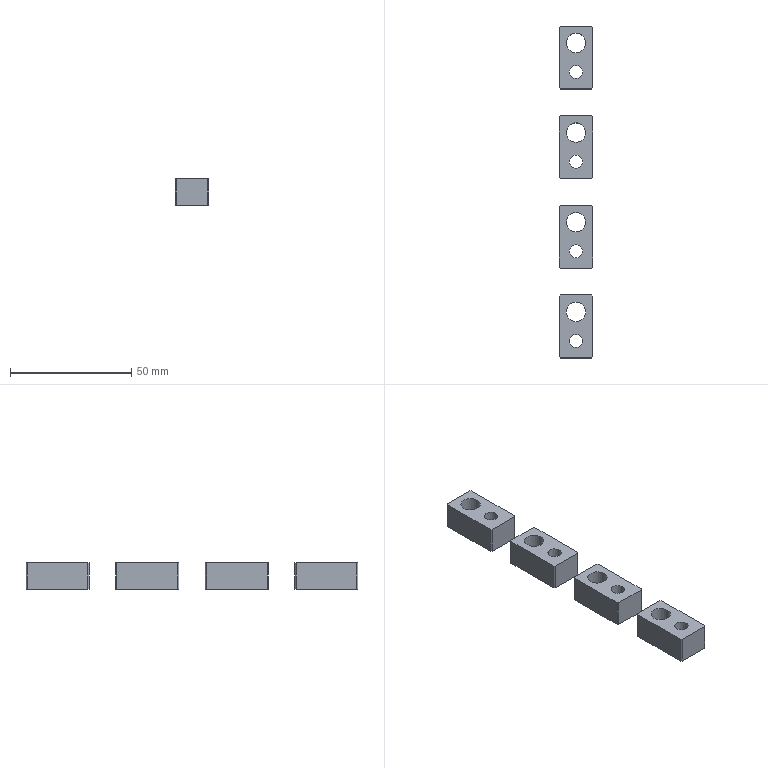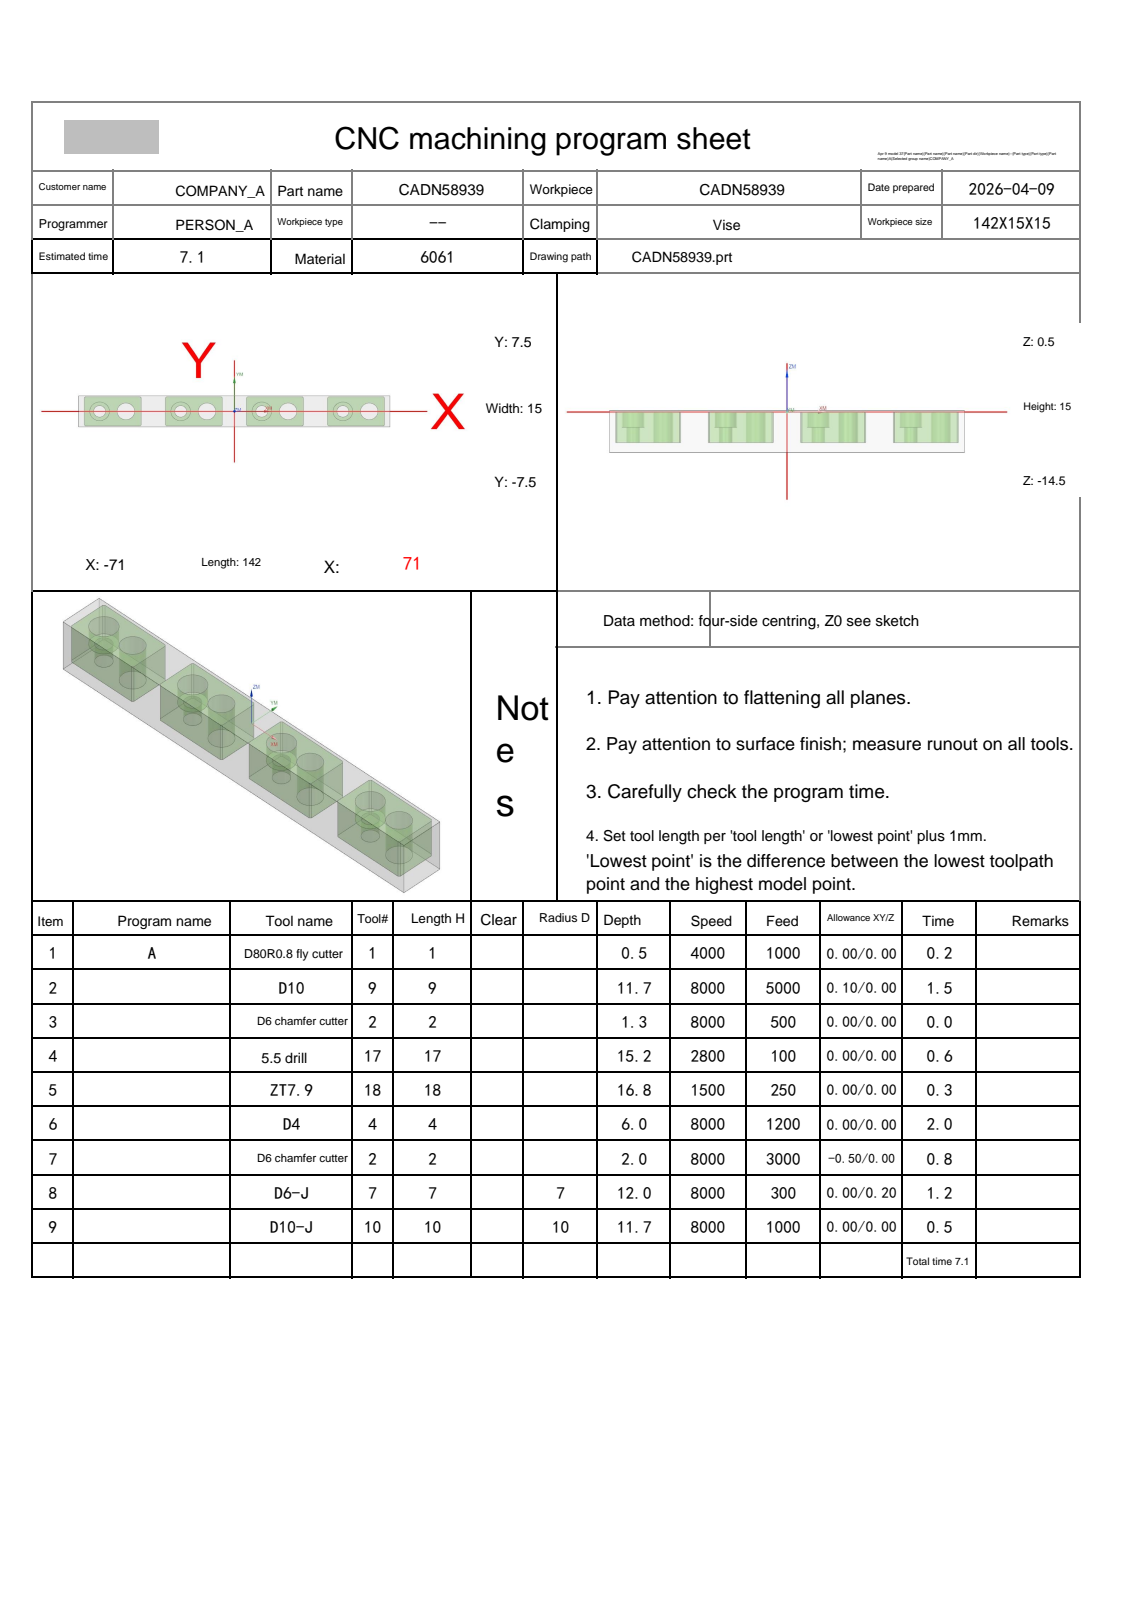NC program | NX | posted by the shop | part box 14 x 137 x 11 mm
Lines 1841 to 2072 of 2072:
N8 T07 M06
(D6-J  D=6. R=0. H=07 ce=0.00 di=0.20)
G00 G90 G54 X-12.5 Y0.0 M03 S8000
G43 H07 Z20.
M08
Z.5
G41 D07
G01 X-12.315 Y.077 F300.
G03 X-12.02 Y.52 I-.185 J.443
X-12.5 Y1. I-.48 J0.0
X-12.5 Y1. Z-.5 I0.0 J-1.
X-12.5 Y1. Z-1.5 I0.0 J-1.
X-12.5 Y1. Z-2.5 I0.0 J-1.
X-12.5 Y1. Z-3.5 I0.0 J-1.
X-12.5 Y1. Z-4.5 I0.0 J-1.
X-12.5 Y1. Z-5.5 I0.0 J-1.
X-12.5 Y1. Z-6.5 I0.0 J-1.
X-12.5 Y1. Z-7.5 I0.0 J-1.
X-12.5 Y1. Z-8.5 I0.0 J-1.
X-12.5 Y1. Z-9.5 I0.0 J-1.
X-12.5 Y1. Z-10.5 I0.0 J-1.
X-12.5 Y1. Z-11.5 I0.0 J-1.
X-13.5 Y0.0 I0.0 J-1.
X-12.5 Y-1. I1. J0.0
X-11.5 Y0.0 I0.0 J1.
X-12.5 Y1. I-1. J0.0
X-12.98 Y.52 I0.0 J-.48
X-12.685 Y.077 I.48 J0.0
G01 G40 X-12.5 Y0.0
G00 Z20.
X-49.5
Z.5
G41 D07
G01 X-49.315 Y.077
G03 X-49.02 Y.52 I-.185 J.443
X-49.5 Y1. I-.48 J0.0
X-49.5 Y1. Z-.5 I0.0 J-1.
X-49.5 Y1. Z-1.5 I0.0 J-1.
X-49.5 Y1. Z-2.5 I0.0 J-1.
X-49.5 Y1. Z-3.5 I0.0 J-1.
X-49.5 Y1. Z-4.5 I0.0 J-1.
X-49.5 Y1. Z-5.5 I0.0 J-1.
X-49.5 Y1. Z-6.5 I0.0 J-1.
X-49.5 Y1. Z-7.5 I0.0 J-1.
X-49.5 Y1. Z-8.5 I0.0 J-1.
X-49.5 Y1. Z-9.5 I0.0 J-1.
X-49.5 Y1. Z-10.5 I0.0 J-1.
X-49.5 Y1. Z-11.5 I0.0 J-1.
X-50.5 Y0.0 I0.0 J-1.
X-49.5 Y-1. I1. J0.0
X-48.5 Y0.0 I0.0 J1.
X-49.5 Y1. I-1. J0.0
X-49.98 Y.52 I0.0 J-.48
X-49.685 Y.077 I.48 J0.0
G01 G40 X-49.5 Y0.0
G00 Z20.
X24.5
Z.5
G41 D07
G01 X24.685 Y.077
G03 X24.98 Y.52 I-.185 J.443
X24.5 Y1. I-.48 J0.0
X24.5 Y1. Z-.5 I0.0 J-1.
X24.5 Y1. Z-1.5 I0.0 J-1.
X24.5 Y1. Z-2.5 I0.0 J-1.
X24.5 Y1. Z-3.5 I0.0 J-1.
X24.5 Y1. Z-4.5 I0.0 J-1.
X24.5 Y1. Z-5.5 I0.0 J-1.
X24.5 Y1. Z-6.5 I0.0 J-1.
X24.5 Y1. Z-7.5 I0.0 J-1.
X24.5 Y1. Z-8.5 I0.0 J-1.
X24.5 Y1. Z-9.5 I0.0 J-1.
X24.5 Y1. Z-10.5 I0.0 J-1.
X24.5 Y1. Z-11.5 I0.0 J-1.
X23.5 Y0.0 I0.0 J-1.
X24.5 Y-1. I1. J0.0
X25.5 Y0.0 I0.0 J1.
X24.5 Y1. I-1. J0.0
X24.02 Y.52 I0.0 J-.48
X24.315 Y.077 I.48 J0.0
G01 G40 X24.5 Y0.0
G00 Z20.
X61.5
Z.5
G41 D07
G01 X61.685 Y.077
G03 X61.98 Y.52 I-.185 J.443
X61.5 Y1. I-.48 J0.0
X61.5 Y1. Z-.5 I0.0 J-1.
X61.5 Y1. Z-1.5 I0.0 J-1.
X61.5 Y1. Z-2.5 I0.0 J-1.
X61.5 Y1. Z-3.5 I0.0 J-1.
X61.5 Y1. Z-4.5 I0.0 J-1.
X61.5 Y1. Z-5.5 I0.0 J-1.
X61.5 Y1. Z-6.5 I0.0 J-1.
X61.5 Y1. Z-7.5 I0.0 J-1.
X61.5 Y1. Z-8.5 I0.0 J-1.
X61.5 Y1. Z-9.5 I0.0 J-1.
X61.5 Y1. Z-10.5 I0.0 J-1.
X61.5 Y1. Z-11.5 I0.0 J-1.
X60.5 Y0.0 I0.0 J-1.
X61.5 Y-1. I1. J0.0
X62.5 Y0.0 I0.0 J1.
X61.5 Y1. I-1. J0.0
X61.02 Y.52 I0.0 J-.48
X61.315 Y.077 I.48 J0.0
G01 G40 X61.5 Y0.0
G00 Z20.
G91 G28 Z0.0
M05
M09
G91 G28 Z0.0
M01
N9 T10 M06
(D10-J  D=10. R=0. H=10 ce=0.00 di=0.00)
G00 G90 G54 X-41.987 Y-13.116 M03 S8000
G43 H10 Z20.
M08
Z-10.7
G01 Z-11.2 F1000.
G41 D10
X-42.003 Y-12.917
G03 X-43. Y-12. I-.997 J-.083
G01 X-68.
G02 X-71.536 Y-10.536 I0.0 J5.
G01 X-72.036 Y-10.036
G02 X-73.5 Y-6.5 I3.536 J3.536
G01 Y6.5
G02 X-72.036 Y10.036 I5. J0.0
G01 X-71.536 Y10.536
G02 X-68. Y12. I3.536 J-3.536
G01 X-43.
G02 X-39.464 Y10.536 I0.0 J-5.
G01 X-38.964 Y10.036
G02 X-37.5 Y6.5 I-3.536 J-3.536
G01 Y-6.5
G02 X-38.964 Y-10.036 I-5. J0.0
G01 X-39.464 Y-10.536
G02 X-43. Y-12. I-3.536 J3.536
G01 X-43.5
G03 X-44.5 Y-13. I0.0 J-1.
G01 G40 Y-13.2
X-36.58 Y-10.053
G41 D10
X-36.408 Y-9.952
G03 X-35.913 Y-9.089 I-.505 J.863
X-36.011 Y-8.657 I-1. J0.0
G02 X-36.5 Y-6.5 I4.511 J2.157
G01 Y6.5
G02 X-35.036 Y10.036 I5. J0.0
G01 X-34.536 Y10.536
G02 X-31. Y12. I3.536 J-3.536
G01 X-6.
G02 X-2.464 Y10.536 I0.0 J-5.
G01 X-1.964 Y10.036
G02 X-.5 Y6.5 I-3.536 J-3.536
G01 Y-6.5
G02 X-1.964 Y-10.036 I-5. J0.0
G01 X-2.464 Y-10.536
G02 X-6. Y-12. I-3.536 J3.536
G01 X-31.
G02 X-34.536 Y-10.536 I0.0 J5.
G01 X-35.036 Y-10.036
G02 X-36.011 Y-8.657 I3.536 J3.536
X-36.204 Y-8.196 I4.511 J2.157
G03 X-37.144 Y-7.535 I-.941 J-.339
X-37.483 Y-7.595 I0.0 J-1.
G01 G40 X-37. Y-8.898
Z-10.7
G00 Z20.
X17.5 Y13.2
Z-10.7
G01 Z-11.2
G41 D10
Y13.
G03 X18.5 Y12. I1. J0.0
G01 X31.
G02 X34.536 Y10.536 I0.0 J-5.
G01 X35.036 Y10.036
G02 X36.5 Y6.5 I-3.536 J-3.536
G01 Y-6.5
G02 X35.036 Y-10.036 I-5. J0.0
G01 X34.536 Y-10.536
G02 X31. Y-12. I-3.536 J3.536
G01 X6.
G02 X2.464 Y-10.536 I0.0 J5.
G01 X1.964 Y-10.036
G02 X.5 Y-6.5 I3.536 J3.536
G01 Y6.5
G02 X1.964 Y10.036 I5. J0.0
G01 X2.464 Y10.536
G02 X6. Y12. I3.536 J-3.536
G01 X18.5
X19.
G03 X20. Y13. I0.0 J1.
G01 G40 Y13.2
Z-10.7
G00 Z20.
X54.5
Z-10.7
G01 Z-11.2
G41 D10
Y13.
G03 X55.5 Y12. I1. J0.0
G01 X68.
G02 X71.536 Y10.536 I0.0 J-5.
G01 X72.036 Y10.036
G02 X73.5 Y6.5 I-3.536 J-3.536
G01 Y-6.5
G02 X72.036 Y-10.036 I-5. J0.0
G01 X71.536 Y-10.536
G02 X68. Y-12. I-3.536 J3.536
G01 X43.
G02 X39.464 Y-10.536 I0.0 J5.
G01 X38.964 Y-10.036
G02 X37.5 Y-6.5 I3.536 J3.536
G01 Y6.5
G02 X38.964 Y10.036 I5. J0.0
G01 X39.464 Y10.536
G02 X43. Y12. I3.536 J-3.536
G01 X55.5
X56.
G03 X57. Y13. I0.0 J1.
G01 G40 Y13.2
Z-10.7
G00 Z20.
M05
M09
G91 G28 Z0.0
G91 G28 Y0.0
M30
%